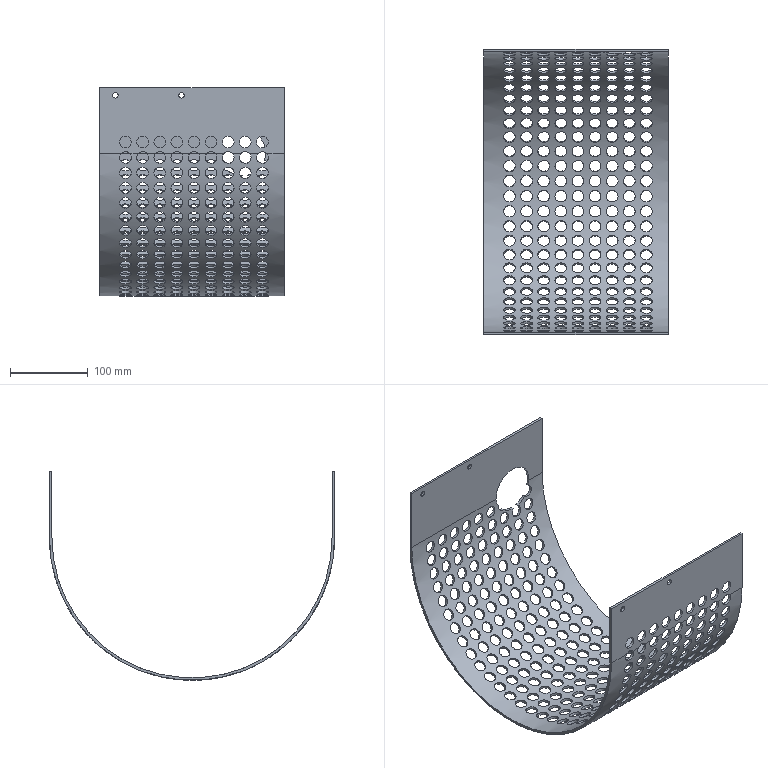Part | STEP file | 40A-00290-78-01 | 1 solid | 578 faces | box 237 x 366.4 x 268.2 mm | volume 401444 mm3 | spline 539 | cylinder 31 | plane 8 | commonest cylinder face diameters 15 x18 7 x8 60 x3 360 x1 366.4 x1